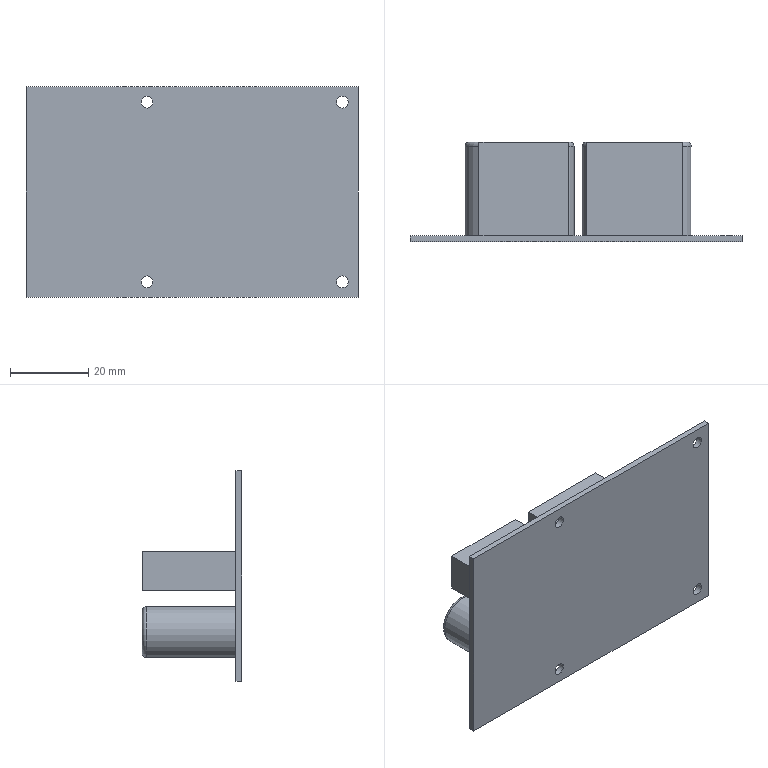Part | STEP file | 6151212W | 1 solid | 42 faces | box 85 x 25.5 x 54 mm | volume 22602 mm3 | plane 30 | cylinder 8 | torus 4 | commonest cylinder face diameters 3 x4 13 x4
STEP:
#1=CARTESIAN_POINT('',(8.051,1.5,-7.857));
#2=VERTEX_POINT('',#1);
#3=CARTESIAN_POINT('',(8.051,1.5,-14.357));
#4=DIRECTION('',(0.,1.,0.));
#5=DIRECTION('',(0.,0.,1.));
#6=AXIS2_PLACEMENT_3D('',#3,#4,#5);
#7=CIRCLE('',#6,6.5);
#8=EDGE_CURVE('',#2,#2,#7,.T.);
#9=ORIENTED_EDGE('',*,*,#8,.F.);
#10=EDGE_LOOP('',(#9));
#11=FACE_BOUND('',#10,.T.);
#12=CARTESIAN_POINT('',(-24.841,1.5,6.301));
#13=VERTEX_POINT('',#12);
#14=CARTESIAN_POINT('',(-1.911,1.5,6.301));
#15=VERTEX_POINT('',#14);
#16=CARTESIAN_POINT('',(-24.841,1.5,6.301));
#17=DIRECTION('',(1.,0.,0.));
#18=VECTOR('',#17,1000.);
#19=LINE('',#16,#18);
#20=EDGE_CURVE('',#13,#15,#19,.T.);
#21=ORIENTED_EDGE('',*,*,#20,.F.);
#22=CARTESIAN_POINT('',(-24.841,1.5,-3.718));
#23=VERTEX_POINT('',#22);
#24=CARTESIAN_POINT('',(-24.841,1.5,-3.718));
#25=DIRECTION('',(0.,0.,1.));
#26=VECTOR('',#25,1000.);
#27=LINE('',#24,#26);
#28=EDGE_CURVE('',#23,#13,#27,.T.);
#29=ORIENTED_EDGE('',*,*,#28,.F.);
#30=CARTESIAN_POINT('',(-1.911,1.5,-3.718));
#31=VERTEX_POINT('',#30);
#32=CARTESIAN_POINT('',(-24.841,1.5,-3.718));
#33=DIRECTION('',(-1.,0.,0.));
#34=VECTOR('',#33,1000.);
#35=LINE('',#32,#34);
#36=EDGE_CURVE('',#31,#23,#35,.T.);
#37=ORIENTED_EDGE('',*,*,#36,.F.);
#38=CARTESIAN_POINT('',(-1.911,1.5,-3.718));
#39=DIRECTION('',(0.,0.,-1.));
#40=VECTOR('',#39,1000.);
#41=LINE('',#38,#40);
#42=EDGE_CURVE('',#15,#31,#41,.T.);
#43=ORIENTED_EDGE('',*,*,#42,.F.);
#44=EDGE_LOOP('',(#21,#29,#37,#43));
#45=FACE_BOUND('',#44,.T.);
#46=CARTESIAN_POINT('',(-21.949,1.5,-7.857));
#47=VERTEX_POINT('',#46);
#48=CARTESIAN_POINT('',(-21.949,1.5,-14.357));
#49=DIRECTION('',(0.,1.,0.));
#50=DIRECTION('',(0.,0.,1.));
#51=AXIS2_PLACEMENT_3D('',#48,#49,#50);
#52=CIRCLE('',#51,6.5);
#53=EDGE_CURVE('',#47,#47,#52,.T.);
#54=ORIENTED_EDGE('',*,*,#53,.F.);
#55=EDGE_LOOP('',(#54));
#56=FACE_BOUND('',#55,.T.);
#57=CARTESIAN_POINT('',(38.5,1.5,21.5));
#58=VERTEX_POINT('',#57);
#59=CARTESIAN_POINT('',(38.5,1.5,23.));
#60=DIRECTION('',(0.,1.,0.));
#61=DIRECTION('',(0.,0.,-1.));
#62=AXIS2_PLACEMENT_3D('',#59,#60,#61);
#63=CIRCLE('',#62,1.5);
#64=EDGE_CURVE('',#58,#58,#63,.T.);
#65=ORIENTED_EDGE('',*,*,#64,.F.);
#66=EDGE_LOOP('',(#65));
#67=FACE_BOUND('',#66,.T.);
#68=CARTESIAN_POINT('',(-11.5,1.5,-21.5));
#69=VERTEX_POINT('',#68);
#70=CARTESIAN_POINT('',(-11.5,1.5,-23.));
#71=DIRECTION('',(0.,1.,0.));
#72=DIRECTION('',(0.,0.,1.));
#73=AXIS2_PLACEMENT_3D('',#70,#71,#72);
#74=CIRCLE('',#73,1.5);
#75=EDGE_CURVE('',#69,#69,#74,.T.);
#76=ORIENTED_EDGE('',*,*,#75,.F.);
#77=EDGE_LOOP('',(#76));
#78=FACE_BOUND('',#77,.T.);
#79=CARTESIAN_POINT('',(-42.5,1.5,-27.));
#80=VERTEX_POINT('',#79);
#81=CARTESIAN_POINT('',(-42.5,1.5,27.));
#82=VERTEX_POINT('',#81);
#83=CARTESIAN_POINT('',(-42.5,1.5,-27.));
#84=DIRECTION('',(0.,0.,1.));
#85=VECTOR('',#84,1000.);
#86=LINE('',#83,#85);
#87=EDGE_CURVE('',#80,#82,#86,.T.);
#88=ORIENTED_EDGE('',*,*,#87,.T.);
#89=CARTESIAN_POINT('',(42.5,1.5,27.));
#90=VERTEX_POINT('',#89);
#91=CARTESIAN_POINT('',(-42.5,1.5,27.));
#92=DIRECTION('',(1.,0.,0.));
#93=VECTOR('',#92,1000.);
#94=LINE('',#91,#93);
#95=EDGE_CURVE('',#82,#90,#94,.T.);
#96=ORIENTED_EDGE('',*,*,#95,.T.);
#97=CARTESIAN_POINT('',(42.5,1.5,-27.));
#98=VERTEX_POINT('',#97);
#99=CARTESIAN_POINT('',(42.5,1.5,-27.));
#100=DIRECTION('',(0.,0.,-1.));
#101=VECTOR('',#100,1000.);
#102=LINE('',#99,#101);
#103=EDGE_CURVE('',#90,#98,#102,.T.);
#104=ORIENTED_EDGE('',*,*,#103,.T.);
#105=CARTESIAN_POINT('',(-42.5,1.5,-27.));
#106=DIRECTION('',(-1.,0.,0.));
#107=VECTOR('',#106,1000.);
#108=LINE('',#105,#107);
#109=EDGE_CURVE('',#98,#80,#108,.T.);
#110=ORIENTED_EDGE('',*,*,#109,.T.);
#111=EDGE_LOOP('',(#88,#96,#104,#110));
#112=FACE_OUTER_BOUND('',#111,.T.);
#113=CARTESIAN_POINT('',(-11.5,1.5,24.5));
#114=VERTEX_POINT('',#113);
#115=CARTESIAN_POINT('',(-11.5,1.5,23.));
#116=DIRECTION('',(0.,1.,0.));
#117=DIRECTION('',(0.,0.,1.));
#118=AXIS2_PLACEMENT_3D('',#115,#116,#117);
#119=CIRCLE('',#118,1.5);
#120=EDGE_CURVE('',#114,#114,#119,.T.);
#121=ORIENTED_EDGE('',*,*,#120,.F.);
#122=EDGE_LOOP('',(#121));
#123=FACE_BOUND('',#122,.T.);
#124=CARTESIAN_POINT('',(38.5,1.5,-24.5));
#125=VERTEX_POINT('',#124);
#126=CARTESIAN_POINT('',(38.5,1.5,-23.));
#127=DIRECTION('',(0.,1.,0.));
#128=DIRECTION('',(0.,0.,-1.));
#129=AXIS2_PLACEMENT_3D('',#126,#127,#128);
#130=CIRCLE('',#129,1.5);
#131=EDGE_CURVE('',#125,#125,#130,.T.);
#132=ORIENTED_EDGE('',*,*,#131,.F.);
#133=EDGE_LOOP('',(#132));
#134=FACE_BOUND('',#133,.T.);
#135=CARTESIAN_POINT('',(-6.949,1.5,-7.857));
#136=VERTEX_POINT('',#135);
#137=CARTESIAN_POINT('',(-6.949,1.5,-14.357));
#138=DIRECTION('',(0.,1.,0.));
#139=DIRECTION('',(0.,0.,1.));
#140=AXIS2_PLACEMENT_3D('',#137,#138,#139);
#141=CIRCLE('',#140,6.5);
#142=EDGE_CURVE('',#136,#136,#141,.T.);
#143=ORIENTED_EDGE('',*,*,#142,.F.);
#144=EDGE_LOOP('',(#143));
#145=FACE_BOUND('',#144,.T.);
#146=CARTESIAN_POINT('',(23.051,1.5,-7.857));
#147=VERTEX_POINT('',#146);
#148=CARTESIAN_POINT('',(23.051,1.5,-14.357));
#149=DIRECTION('',(0.,1.,0.));
#150=DIRECTION('',(0.,0.,1.));
#151=AXIS2_PLACEMENT_3D('',#148,#149,#150);
#152=CIRCLE('',#151,6.5);
#153=EDGE_CURVE('',#147,#147,#152,.T.);
#154=ORIENTED_EDGE('',*,*,#153,.F.);
#155=EDGE_LOOP('',(#154));
#156=FACE_BOUND('',#155,.T.);
#157=CARTESIAN_POINT('',(2.737,1.5,6.301));
#158=VERTEX_POINT('',#157);
#159=CARTESIAN_POINT('',(27.32,1.5,6.301));
#160=VERTEX_POINT('',#159);
#161=CARTESIAN_POINT('',(2.737,1.5,6.301));
#162=DIRECTION('',(1.,0.,0.));
#163=VECTOR('',#162,1000.);
#164=LINE('',#161,#163);
#165=EDGE_CURVE('',#158,#160,#164,.T.);
#166=ORIENTED_EDGE('',*,*,#165,.F.);
#167=CARTESIAN_POINT('',(2.737,1.5,-3.718));
#168=VERTEX_POINT('',#167);
#169=CARTESIAN_POINT('',(2.737,1.5,-3.718));
#170=DIRECTION('',(0.,0.,1.));
#171=VECTOR('',#170,1000.);
#172=LINE('',#169,#171);
#173=EDGE_CURVE('',#168,#158,#172,.T.);
#174=ORIENTED_EDGE('',*,*,#173,.F.);
#175=CARTESIAN_POINT('',(27.32,1.5,-3.718));
#176=VERTEX_POINT('',#175);
#177=CARTESIAN_POINT('',(2.737,1.5,-3.718));
#178=DIRECTION('',(-1.,0.,0.));
#179=VECTOR('',#178,1000.);
#180=LINE('',#177,#179);
#181=EDGE_CURVE('',#176,#168,#180,.T.);
#182=ORIENTED_EDGE('',*,*,#181,.F.);
#183=CARTESIAN_POINT('',(27.32,1.5,-3.718));
#184=DIRECTION('',(0.,0.,-1.));
#185=VECTOR('',#184,1000.);
#186=LINE('',#183,#185);
#187=EDGE_CURVE('',#160,#176,#186,.T.);
#188=ORIENTED_EDGE('',*,*,#187,.F.);
#189=EDGE_LOOP('',(#166,#174,#182,#188));
#190=FACE_BOUND('',#189,.T.);
#191=CARTESIAN_POINT('',(-42.5,1.5,-27.));
#192=DIRECTION('',(0.,1.,0.));
#193=DIRECTION('',(0.,0.,1.));
#194=AXIS2_PLACEMENT_3D('',#191,#192,#193);
#195=PLANE('',#194);
#196=ADVANCED_FACE('',(#11,#45,#56,#67,#78,#112,#123,#134,#145,#156,#190),#195,.T.);
#197=CARTESIAN_POINT('',(38.5,0.,21.5));
#198=VERTEX_POINT('',#197);
#199=CARTESIAN_POINT('',(38.5,0.,23.));
#200=DIRECTION('',(0.,1.,0.));
#201=DIRECTION('',(0.,0.,-1.));
#202=AXIS2_PLACEMENT_3D('',#199,#200,#201);
#203=CIRCLE('',#202,1.5);
#204=EDGE_CURVE('',#198,#198,#203,.T.);
#205=ORIENTED_EDGE('',*,*,#204,.T.);
#206=EDGE_LOOP('',(#205));
#207=FACE_BOUND('',#206,.T.);
#208=CARTESIAN_POINT('',(-11.5,0.,-21.5));
#209=VERTEX_POINT('',#208);
#210=CARTESIAN_POINT('',(-11.5,0.,-23.));
#211=DIRECTION('',(0.,1.,0.));
#212=DIRECTION('',(0.,0.,1.));
#213=AXIS2_PLACEMENT_3D('',#210,#211,#212);
#214=CIRCLE('',#213,1.5);
#215=EDGE_CURVE('',#209,#209,#214,.T.);
#216=ORIENTED_EDGE('',*,*,#215,.T.);
#217=EDGE_LOOP('',(#216));
#218=FACE_BOUND('',#217,.T.);
#219=CARTESIAN_POINT('',(-42.5,0.,-27.));
#220=VERTEX_POINT('',#219);
#221=CARTESIAN_POINT('',(-42.5,0.,27.));
#222=VERTEX_POINT('',#221);
#223=CARTESIAN_POINT('',(-42.5,0.,-27.));
#224=DIRECTION('',(0.,0.,1.));
#225=VECTOR('',#224,1000.);
#226=LINE('',#223,#225);
#227=EDGE_CURVE('',#220,#222,#226,.T.);
#228=ORIENTED_EDGE('',*,*,#227,.F.);
#229=CARTESIAN_POINT('',(42.5,0.,-27.));
#230=VERTEX_POINT('',#229);
#231=CARTESIAN_POINT('',(-42.5,0.,-27.));
#232=DIRECTION('',(-1.,0.,0.));
#233=VECTOR('',#232,1000.);
#234=LINE('',#231,#233);
#235=EDGE_CURVE('',#230,#220,#234,.T.);
#236=ORIENTED_EDGE('',*,*,#235,.F.);
#237=CARTESIAN_POINT('',(42.5,0.,27.));
#238=VERTEX_POINT('',#237);
#239=CARTESIAN_POINT('',(42.5,0.,-27.));
#240=DIRECTION('',(0.,0.,-1.));
#241=VECTOR('',#240,1000.);
#242=LINE('',#239,#241);
#243=EDGE_CURVE('',#238,#230,#242,.T.);
#244=ORIENTED_EDGE('',*,*,#243,.F.);
#245=CARTESIAN_POINT('',(-42.5,0.,27.));
#246=DIRECTION('',(1.,0.,0.));
#247=VECTOR('',#246,1000.);
#248=LINE('',#245,#247);
#249=EDGE_CURVE('',#222,#238,#248,.T.);
#250=ORIENTED_EDGE('',*,*,#249,.F.);
#251=EDGE_LOOP('',(#228,#236,#244,#250));
#252=FACE_OUTER_BOUND('',#251,.T.);
#253=CARTESIAN_POINT('',(-11.5,0.,24.5));
#254=VERTEX_POINT('',#253);
#255=CARTESIAN_POINT('',(-11.5,0.,23.));
#256=DIRECTION('',(0.,1.,0.));
#257=DIRECTION('',(0.,0.,1.));
#258=AXIS2_PLACEMENT_3D('',#255,#256,#257);
#259=CIRCLE('',#258,1.5);
#260=EDGE_CURVE('',#254,#254,#259,.T.);
#261=ORIENTED_EDGE('',*,*,#260,.T.);
#262=EDGE_LOOP('',(#261));
#263=FACE_BOUND('',#262,.T.);
#264=CARTESIAN_POINT('',(38.5,0.,-24.5));
#265=VERTEX_POINT('',#264);
#266=CARTESIAN_POINT('',(38.5,0.,-23.));
#267=DIRECTION('',(0.,1.,0.));
#268=DIRECTION('',(0.,0.,-1.));
#269=AXIS2_PLACEMENT_3D('',#266,#267,#268);
#270=CIRCLE('',#269,1.5);
#271=EDGE_CURVE('',#265,#265,#270,.T.);
#272=ORIENTED_EDGE('',*,*,#271,.T.);
#273=EDGE_LOOP('',(#272));
#274=FACE_BOUND('',#273,.T.);
#275=CARTESIAN_POINT('',(-42.5,0.,-27.));
#276=DIRECTION('',(0.,1.,0.));
#277=DIRECTION('',(0.,0.,1.));
#278=AXIS2_PLACEMENT_3D('',#275,#276,#277);
#279=PLANE('',#278);
#280=ADVANCED_FACE('',(#207,#218,#252,#263,#274),#279,.F.);
#281=ORIENTED_EDGE('',*,*,#227,.T.);
#282=CARTESIAN_POINT('',(-42.5,1.5,27.));
#283=DIRECTION('',(0.,-1.,0.));
#284=VECTOR('',#283,1000.);
#285=LINE('',#282,#284);
#286=EDGE_CURVE('',#82,#222,#285,.T.);
#287=ORIENTED_EDGE('',*,*,#286,.F.);
#288=ORIENTED_EDGE('',*,*,#87,.F.);
#289=CARTESIAN_POINT('',(-42.5,1.5,-27.));
#290=DIRECTION('',(0.,-1.,0.));
#291=VECTOR('',#290,1000.);
#292=LINE('',#289,#291);
#293=EDGE_CURVE('',#80,#220,#292,.T.);
#294=ORIENTED_EDGE('',*,*,#293,.T.);
#295=EDGE_LOOP('',(#281,#287,#288,#294));
#296=FACE_OUTER_BOUND('',#295,.T.);
#297=CARTESIAN_POINT('',(-42.5,1.5,-27.));
#298=DIRECTION('',(1.,0.,0.));
#299=DIRECTION('',(0.,0.,-1.));
#300=AXIS2_PLACEMENT_3D('',#297,#298,#299);
#301=PLANE('',#300);
#302=ADVANCED_FACE('',(#296),#301,.F.);
#303=ORIENTED_EDGE('',*,*,#249,.T.);
#304=CARTESIAN_POINT('',(42.5,1.5,27.));
#305=DIRECTION('',(0.,-1.,0.));
#306=VECTOR('',#305,1000.);
#307=LINE('',#304,#306);
#308=EDGE_CURVE('',#90,#238,#307,.T.);
#309=ORIENTED_EDGE('',*,*,#308,.F.);
#310=ORIENTED_EDGE('',*,*,#95,.F.);
#311=ORIENTED_EDGE('',*,*,#286,.T.);
#312=EDGE_LOOP('',(#303,#309,#310,#311));
#313=FACE_OUTER_BOUND('',#312,.T.);
#314=CARTESIAN_POINT('',(-42.5,1.5,27.));
#315=DIRECTION('',(0.,0.,-1.));
#316=DIRECTION('',(-1.,0.,0.));
#317=AXIS2_PLACEMENT_3D('',#314,#315,#316);
#318=PLANE('',#317);
#319=ADVANCED_FACE('',(#313),#318,.F.);
#320=ORIENTED_EDGE('',*,*,#243,.T.);
#321=CARTESIAN_POINT('',(42.5,1.5,-27.));
#322=DIRECTION('',(0.,-1.,0.));
#323=VECTOR('',#322,1000.);
#324=LINE('',#321,#323);
#325=EDGE_CURVE('',#98,#230,#324,.T.);
#326=ORIENTED_EDGE('',*,*,#325,.F.);
#327=ORIENTED_EDGE('',*,*,#103,.F.);
#328=ORIENTED_EDGE('',*,*,#308,.T.);
#329=EDGE_LOOP('',(#320,#326,#327,#328));
#330=FACE_OUTER_BOUND('',#329,.T.);
#331=CARTESIAN_POINT('',(42.5,1.5,-27.));
#332=DIRECTION('',(-1.,0.,0.));
#333=DIRECTION('',(0.,0.,1.));
#334=AXIS2_PLACEMENT_3D('',#331,#332,#333);
#335=PLANE('',#334);
#336=ADVANCED_FACE('',(#330),#335,.F.);
#337=ORIENTED_EDGE('',*,*,#235,.T.);
#338=ORIENTED_EDGE('',*,*,#293,.F.);
#339=ORIENTED_EDGE('',*,*,#109,.F.);
#340=ORIENTED_EDGE('',*,*,#325,.T.);
#341=EDGE_LOOP('',(#337,#338,#339,#340));
#342=FACE_OUTER_BOUND('',#341,.T.);
#343=CARTESIAN_POINT('',(-42.5,1.5,-27.));
#344=DIRECTION('',(0.,0.,1.));
#345=DIRECTION('',(1.,0.,0.));
#346=AXIS2_PLACEMENT_3D('',#343,#344,#345);
#347=PLANE('',#346);
#348=ADVANCED_FACE('',(#342),#347,.F.);
#349=ORIENTED_EDGE('',*,*,#75,.T.);
#350=EDGE_LOOP('',(#349));
#351=FACE_OUTER_BOUND('',#350,.T.);
#352=ORIENTED_EDGE('',*,*,#215,.F.);
#353=EDGE_LOOP('',(#352));
#354=FACE_OUTER_BOUND('',#353,.T.);
#355=CARTESIAN_POINT('',(-11.5,1.5,-23.));
#356=DIRECTION('',(0.,-1.,0.));
#357=DIRECTION('',(0.,0.,-1.));
#358=AXIS2_PLACEMENT_3D('',#355,#356,#357);
#359=CYLINDRICAL_SURFACE('',#358,1.5);
#360=ADVANCED_FACE('',(#351,#354),#359,.F.);
#361=ORIENTED_EDGE('',*,*,#120,.T.);
#362=EDGE_LOOP('',(#361));
#363=FACE_OUTER_BOUND('',#362,.T.);
#364=ORIENTED_EDGE('',*,*,#260,.F.);
#365=EDGE_LOOP('',(#364));
#366=FACE_OUTER_BOUND('',#365,.T.);
#367=CARTESIAN_POINT('',(-11.5,1.5,23.));
#368=DIRECTION('',(0.,-1.,0.));
#369=DIRECTION('',(0.,0.,-1.));
#370=AXIS2_PLACEMENT_3D('',#367,#368,#369);
#371=CYLINDRICAL_SURFACE('',#370,1.5);
#372=ADVANCED_FACE('',(#363,#366),#371,.F.);
#373=ORIENTED_EDGE('',*,*,#64,.T.);
#374=EDGE_LOOP('',(#373));
#375=FACE_OUTER_BOUND('',#374,.T.);
#376=ORIENTED_EDGE('',*,*,#204,.F.);
#377=EDGE_LOOP('',(#376));
#378=FACE_OUTER_BOUND('',#377,.T.);
#379=CARTESIAN_POINT('',(38.5,1.5,23.));
#380=DIRECTION('',(0.,-1.,0.));
#381=DIRECTION('',(0.,0.,-1.));
#382=AXIS2_PLACEMENT_3D('',#379,#380,#381);
#383=CYLINDRICAL_SURFACE('',#382,1.5);
#384=ADVANCED_FACE('',(#375,#378),#383,.F.);
#385=ORIENTED_EDGE('',*,*,#131,.T.);
#386=EDGE_LOOP('',(#385));
#387=FACE_OUTER_BOUND('',#386,.T.);
#388=ORIENTED_EDGE('',*,*,#271,.F.);
#389=EDGE_LOOP('',(#388));
#390=FACE_OUTER_BOUND('',#389,.T.);
#391=CARTESIAN_POINT('',(38.5,1.5,-23.));
#392=DIRECTION('',(0.,-1.,0.));
#393=DIRECTION('',(0.,0.,-1.));
#394=AXIS2_PLACEMENT_3D('',#391,#392,#393);
#395=CYLINDRICAL_SURFACE('',#394,1.5);
#396=ADVANCED_FACE('',(#387,#390),#395,.F.);
#397=CARTESIAN_POINT('',(-21.949,24.5,-7.857));
#398=VERTEX_POINT('',#397);
#399=CARTESIAN_POINT('',(-21.949,24.5,-14.357));
#400=DIRECTION('',(0.,-1.,0.));
#401=DIRECTION('',(0.,0.,1.));
#402=AXIS2_PLACEMENT_3D('',#399,#400,#401);
#403=CIRCLE('',#402,6.5);
#404=EDGE_CURVE('',#398,#398,#403,.T.);
#405=ORIENTED_EDGE('',*,*,#404,.T.);
#406=EDGE_LOOP('',(#405));
#407=FACE_OUTER_BOUND('',#406,.T.);
#408=ORIENTED_EDGE('',*,*,#53,.T.);
#409=EDGE_LOOP('',(#408));
#410=FACE_OUTER_BOUND('',#409,.T.);
#411=CARTESIAN_POINT('',(-21.949,25.5,-14.357));
#412=DIRECTION('',(0.,-1.,0.));
#413=DIRECTION('',(0.,0.,-1.));
#414=AXIS2_PLACEMENT_3D('',#411,#412,#413);
#415=CYLINDRICAL_SURFACE('',#414,6.5);
#416=ADVANCED_FACE('',(#407,#410),#415,.T.);
#417=CARTESIAN_POINT('',(-21.949,25.5,-8.857));
#418=VERTEX_POINT('',#417);
#419=CARTESIAN_POINT('',(-21.949,25.5,-14.357));
#420=DIRECTION('',(0.,1.,0.));
#421=DIRECTION('',(0.,0.,1.));
#422=AXIS2_PLACEMENT_3D('',#419,#420,#421);
#423=CIRCLE('',#422,5.5);
#424=EDGE_CURVE('',#418,#418,#423,.T.);
#425=ORIENTED_EDGE('',*,*,#424,.T.);
#426=EDGE_LOOP('',(#425));
#427=FACE_OUTER_BOUND('',#426,.T.);
#428=CARTESIAN_POINT('',(-21.949,25.5,-14.357));
#429=DIRECTION('',(0.,1.,0.));
#430=DIRECTION('',(0.,0.,1.));
#431=AXIS2_PLACEMENT_3D('',#428,#429,#430);
#432=PLANE('',#431);
#433=ADVANCED_FACE('',(#427),#432,.T.);
#434=CARTESIAN_POINT('',(-24.841,25.5,-3.718));
#435=VERTEX_POINT('',#434);
#436=CARTESIAN_POINT('',(-24.841,25.5,6.301));
#437=VERTEX_POINT('',#436);
#438=CARTESIAN_POINT('',(-24.841,25.5,-3.718));
#439=DIRECTION('',(0.,0.,1.));
#440=VECTOR('',#439,1000.);
#441=LINE('',#438,#440);
#442=EDGE_CURVE('',#435,#437,#441,.T.);
#443=ORIENTED_EDGE('',*,*,#442,.T.);
#444=CARTESIAN_POINT('',(-1.911,25.5,6.301));
#445=VERTEX_POINT('',#444);
#446=CARTESIAN_POINT('',(-24.841,25.5,6.301));
#447=DIRECTION('',(1.,0.,0.));
#448=VECTOR('',#447,1000.);
#449=LINE('',#446,#448);
#450=EDGE_CURVE('',#437,#445,#449,.T.);
#451=ORIENTED_EDGE('',*,*,#450,.T.);
#452=CARTESIAN_POINT('',(-1.911,25.5,-3.718));
#453=VERTEX_POINT('',#452);
#454=CARTESIAN_POINT('',(-1.911,25.5,-3.718));
#455=DIRECTION('',(0.,0.,-1.));
#456=VECTOR('',#455,1000.);
#457=LINE('',#454,#456);
#458=EDGE_CURVE('',#445,#453,#457,.T.);
#459=ORIENTED_EDGE('',*,*,#458,.T.);
#460=CARTESIAN_POINT('',(-24.841,25.5,-3.718));
#461=DIRECTION('',(-1.,0.,0.));
#462=VECTOR('',#461,1000.);
#463=LINE('',#460,#462);
#464=EDGE_CURVE('',#453,#435,#463,.T.);
#465=ORIENTED_EDGE('',*,*,#464,.T.);
#466=EDGE_LOOP('',(#443,#451,#459,#465));
#467=FACE_OUTER_BOUND('',#466,.T.);
#468=CARTESIAN_POINT('',(-23.841,25.5,5.301));
#469=VERTEX_POINT('',#468);
#470=CARTESIAN_POINT('',(-2.911,25.5,5.301));
#471=VERTEX_POINT('',#470);
#472=CARTESIAN_POINT('',(-23.841,25.5,5.301));
#473=DIRECTION('',(1.,0.,0.));
#474=VECTOR('',#473,1000.);
#475=LINE('',#472,#474);
#476=EDGE_CURVE('',#469,#471,#475,.T.);
#477=ORIENTED_EDGE('',*,*,#476,.F.);
#478=CARTESIAN_POINT('',(-23.841,25.5,-2.718));
#479=VERTEX_POINT('',#478);
#480=CARTESIAN_POINT('',(-23.841,25.5,-2.718));
#481=DIRECTION('',(0.,0.,1.));
#482=VECTOR('',#481,1000.);
#483=LINE('',#480,#482);
#484=EDGE_CURVE('',#479,#469,#483,.T.);
#485=ORIENTED_EDGE('',*,*,#484,.F.);
#486=CARTESIAN_POINT('',(-2.911,25.5,-2.718));
#487=VERTEX_POINT('',#486);
#488=CARTESIAN_POINT('',(-23.841,25.5,-2.718));
#489=DIRECTION('',(-1.,0.,0.));
#490=VECTOR('',#489,1000.);
#491=LINE('',#488,#490);
#492=EDGE_CURVE('',#487,#479,#491,.T.);
#493=ORIENTED_EDGE('',*,*,#492,.F.);
#494=CARTESIAN_POINT('',(-2.911,25.5,-2.718));
#495=DIRECTION('',(0.,0.,-1.));
#496=VECTOR('',#495,1000.);
#497=LINE('',#494,#496);
#498=EDGE_CURVE('',#471,#487,#497,.T.);
#499=ORIENTED_EDGE('',*,*,#498,.F.);
#500=EDGE_LOOP('',(#477,#485,#493,#499));
#501=FACE_BOUND('',#500,.T.);
#502=CARTESIAN_POINT('',(-24.841,25.5,6.301));
#503=DIRECTION('',(0.,1.,0.));
#504=DIRECTION('',(0.,0.,1.));
#505=AXIS2_PLACEMENT_3D('',#502,#503,#504);
#506=PLANE('',#505);
#507=ADVANCED_FACE('',(#467,#501),#506,.T.);
#508=ORIENTED_EDGE('',*,*,#28,.T.);
#509=CARTESIAN_POINT('',(-24.841,25.5,6.301));
#510=DIRECTION('',(0.,-1.,0.));
#511=VECTOR('',#510,1000.);
#512=LINE('',#509,#511);
#513=EDGE_CURVE('',#437,#13,#512,.T.);
#514=ORIENTED_EDGE('',*,*,#513,.F.);
#515=ORIENTED_EDGE('',*,*,#442,.F.);
#516=CARTESIAN_POINT('',(-24.841,25.5,-3.718));
#517=DIRECTION('',(0.,-1.,0.));
#518=VECTOR('',#517,1000.);
#519=LINE('',#516,#518);
#520=EDGE_CURVE('',#435,#23,#519,.T.);
#521=ORIENTED_EDGE('',*,*,#520,.T.);
#522=EDGE_LOOP('',(#508,#514,#515,#521));
#523=FACE_OUTER_BOUND('',#522,.T.);
#524=CARTESIAN_POINT('',(-24.841,25.5,-3.718));
#525=DIRECTION('',(1.,0.,0.));
#526=DIRECTION('',(0.,0.,-1.));
#527=AXIS2_PLACEMENT_3D('',#524,#525,#526);
#528=PLANE('',#527);
#529=ADVANCED_FACE('',(#523),#528,.F.);
#530=ORIENTED_EDGE('',*,*,#20,.T.);
#531=CARTESIAN_POINT('',(-1.911,25.5,6.301));
#532=DIRECTION('',(0.,-1.,0.));
#533=VECTOR('',#532,1000.);
#534=LINE('',#531,#533);
#535=EDGE_CURVE('',#445,#15,#534,.T.);
#536=ORIENTED_EDGE('',*,*,#535,.F.);
#537=ORIENTED_EDGE('',*,*,#450,.F.);
#538=ORIENTED_EDGE('',*,*,#513,.T.);
#539=EDGE_LOOP('',(#530,#536,#537,#538));
#540=FACE_OUTER_BOUND('',#539,.T.);
#541=CARTESIAN_POINT('',(-24.841,25.5,6.301));
#542=DIRECTION('',(0.,0.,-1.));
#543=DIRECTION('',(-1.,0.,0.));
#544=AXIS2_PLACEMENT_3D('',#541,#542,#543);
#545=PLANE('',#544);
#546=ADVANCED_FACE('',(#540),#545,.F.);
#547=ORIENTED_EDGE('',*,*,#42,.T.);
#548=CARTESIAN_POINT('',(-1.911,25.5,-3.718));
#549=DIRECTION('',(0.,-1.,0.));
#550=VECTOR('',#549,1000.);
#551=LINE('',#548,#550);
#552=EDGE_CURVE('',#453,#31,#551,.T.);
#553=ORIENTED_EDGE('',*,*,#552,.F.);
#554=ORIENTED_EDGE('',*,*,#458,.F.);
#555=ORIENTED_EDGE('',*,*,#535,.T.);
#556=EDGE_LOOP('',(#547,#553,#554,#555));
#557=FACE_OUTER_BOUND('',#556,.T.);
#558=CARTESIAN_POINT('',(-1.911,25.5,-3.718));
#559=DIRECTION('',(-1.,0.,0.));
#560=DIRECTION('',(0.,0.,1.));
#561=AXIS2_PLACEMENT_3D('',#558,#559,#560);
#562=PLANE('',#561);
#563=ADVANCED_FACE('',(#557),#562,.F.);
#564=ORIENTED_EDGE('',*,*,#36,.T.);
#565=ORIENTED_EDGE('',*,*,#520,.F.);
#566=ORIENTED_EDGE('',*,*,#464,.F.);
#567=ORIENTED_EDGE('',*,*,#552,.T.);
#568=EDGE_LOOP('',(#564,#565,#566,#567));
#569=FACE_OUTER_BOUND('',#568,.T.);
#570=CARTESIAN_POINT('',(-24.841,25.5,-3.718));
#571=DIRECTION('',(0.,0.,1.));
#572=DIRECTION('',(1.,0.,0.));
#573=AXIS2_PLACEMENT_3D('',#570,#571,#572);
#574=PLANE('',#573);
#575=ADVANCED_FACE('',(#569),#574,.F.);
#576=CARTESIAN_POINT('',(-23.841,1.5,-2.718));
#577=VERTEX_POINT('',#576);
#578=CARTESIAN_POINT('',(-23.841,1.5,5.301));
#579=VERTEX_POINT('',#578);
#580=CARTESIAN_POINT('',(-23.841,1.5,-2.718));
#581=DIRECTION('',(0.,0.,1.));
#582=VECTOR('',#581,1000.);
#583=LINE('',#580,#582);
#584=EDGE_CURVE('',#577,#579,#583,.T.);
#585=ORIENTED_EDGE('',*,*,#584,.F.);
#586=CARTESIAN_POINT('',(-23.841,25.5,-2.718));
#587=DIRECTION('',(0.,-1.,0.));
#588=VECTOR('',#587,1000.);
#589=LINE('',#586,#588);
#590=EDGE_CURVE('',#479,#577,#589,.T.);
#591=ORIENTED_EDGE('',*,*,#590,.F.);
#592=ORIENTED_EDGE('',*,*,#484,.T.);
#593=CARTESIAN_POINT('',(-23.841,25.5,5.301));
#594=DIRECTION('',(0.,-1.,0.));
#595=VECTOR('',#594,1000.);
#596=LINE('',#593,#595);
#597=EDGE_CURVE('',#469,#579,#596,.T.);
#598=ORIENTED_EDGE('',*,*,#597,.T.);
#599=EDGE_LOOP('',(#585,#591,#592,#598));
#600=FACE_OUTER_BOUND('',#599,.T.);
#601=CARTESIAN_POINT('',(-23.841,25.5,-2.718));
#602=DIRECTION('',(1.,0.,0.));
#603=DIRECTION('',(0.,0.,-1.));
#604=AXIS2_PLACEMENT_3D('',#601,#602,#603);
#605=PLANE('',#604);
#606=ADVANCED_FACE('',(#600),#605,.T.);
#607=CARTESIAN_POINT('',(-2.911,1.5,5.301));
#608=VERTEX_POINT('',#607);
#609=CARTESIAN_POINT('',(-23.841,1.5,5.301));
#610=DIRECTION('',(1.,0.,0.));
#611=VECTOR('',#610,1000.);
#612=LINE('',#609,#611);
#613=EDGE_CURVE('',#579,#608,#612,.T.);
#614=ORIENTED_EDGE('',*,*,#613,.F.);
#615=ORIENTED_EDGE('',*,*,#597,.F.);
#616=ORIENTED_EDGE('',*,*,#476,.T.);
#617=CARTESIAN_POINT('',(-2.911,25.5,5.301));
#618=DIRECTION('',(0.,-1.,0.));
#619=VECTOR('',#618,1000.);
#620=LINE('',#617,#619);
#621=EDGE_CURVE('',#471,#608,#620,.T.);
#622=ORIENTED_EDGE('',*,*,#621,.T.);
#623=EDGE_LOOP('',(#614,#615,#616,#622));
#624=FACE_OUTER_BOUND('',#623,.T.);
#625=CARTESIAN_POINT('',(-23.841,25.5,5.301));
#626=DIRECTION('',(0.,0.,-1.));
#627=DIRECTION('',(-1.,0.,0.));
#628=AXIS2_PLACEMENT_3D('',#625,#626,#627);
#629=PLANE('',#628);
#630=ADVANCED_FACE('',(#624),#629,.T.);
#631=CARTESIAN_POINT('',(-2.911,1.5,-2.718));
#632=VERTEX_POINT('',#631);
#633=CARTESIAN_POINT('',(-2.911,1.5,-2.718));
#634=DIRECTION('',(0.,0.,-1.));
#635=VECTOR('',#634,1000.);
#636=LINE('',#633,#635);
#637=EDGE_CURVE('',#608,#632,#636,.T.);
#638=ORIENTED_EDGE('',*,*,#637,.F.);
#639=ORIENTED_EDGE('',*,*,#621,.F.);
#640=ORIENTED_EDGE('',*,*,#498,.T.);
#641=CARTESIAN_POINT('',(-2.911,25.5,-2.718));
#642=DIRECTION('',(0.,-1.,0.));
#643=VECTOR('',#642,1000.);
#644=LINE('',#641,#643);
#645=EDGE_CURVE('',#487,#632,#644,.T.);
#646=ORIENTED_EDGE('',*,*,#645,.T.);
#647=EDGE_LOOP('',(#638,#639,#640,#646));
#648=FACE_OUTER_BOUND('',#647,.T.);
#649=CARTESIAN_POINT('',(-2.911,25.5,-2.718));
#650=DIRECTION('',(-1.,0.,0.));
#651=DIRECTION('',(0.,0.,1.));
#652=AXIS2_PLACEMENT_3D('',#649,#650,#651);
#653=PLANE('',#652);
#654=ADVANCED_FACE('',(#648),#653,.T.);
#655=CARTESIAN_POINT('',(-23.841,1.5,-2.718));
#656=DIRECTION('',(-1.,0.,0.));
#657=VECTOR('',#656,1000.);
#658=LINE('',#655,#657);
#659=EDGE_CURVE('',#632,#577,#658,.T.);
#660=ORIENTED_EDGE('',*,*,#659,.F.);
#661=ORIENTED_EDGE('',*,*,#645,.F.);
#662=ORIENTED_EDGE('',*,*,#492,.T.);
#663=ORIENTED_EDGE('',*,*,#590,.T.);
#664=EDGE_LOOP('',(#660,#661,#662,#663));
#665=FACE_OUTER_BOUND('',#664,.T.);
#666=CARTESIAN_POINT('',(-23.841,25.5,-2.718));
#667=DIRECTION('',(0.,0.,1.));
#668=DIRECTION('',(1.,0.,0.));
#669=AXIS2_PLACEMENT_3D('',#666,#667,#668);
#670=PLANE('',#669);
#671=ADVANCED_FACE('',(#665),#670,.T.);
#672=ORIENTED_EDGE('',*,*,#584,.T.);
#673=ORIENTED_EDGE('',*,*,#613,.T.);
#674=ORIENTED_EDGE('',*,*,#637,.T.);
#675=ORIENTED_EDGE('',*,*,#659,.T.);
#676=EDGE_LOOP('',(#672,#673,#674,#675));
#677=FACE_OUTER_BOUND('',#676,.T.);
#678=CARTESIAN_POINT('',(-42.5,1.5,-27.));
#679=DIRECTION('',(0.,1.,0.));
#680=DIRECTION('',(0.,0.,1.));
#681=AXIS2_PLACEMENT_3D('',#678,#679,#680);
#682=PLANE('',#681);
#683=ADVANCED_FACE('',(#677),#682,.T.);
#684=CARTESIAN_POINT('',(-6.949,24.5,-7.857));
#685=VERTEX_POINT('',#684);
#686=CARTESIAN_POINT('',(-6.949,24.5,-14.357));
#687=DIRECTION('',(0.,-1.,0.));
#688=DIRECTION('',(0.,0.,1.));
#689=AXIS2_PLACEMENT_3D('',#686,#687,#688);
#690=CIRCLE('',#689,6.5);
#691=EDGE_CURVE('',#685,#685,#690,.T.);
#692=ORIENTED_EDGE('',*,*,#691,.T.);
#693=EDGE_LOOP('',(#692));
#694=FACE_OUTER_BOUND('',#693,.T.);
#695=ORIENTED_EDGE('',*,*,#142,.T.);
#696=EDGE_LOOP('',(#695));
#697=FACE_OUTER_BOUND('',#696,.T.);
#698=CARTESIAN_POINT('',(-6.949,25.5,-14.357));
#699=DIRECTION('',(0.,-1.,0.));
#700=DIRECTION('',(0.,0.,-1.));
#701=AXIS2_PLACEMENT_3D('',#698,#699,#700);
#702=CYLINDRICAL_SURFACE('',#701,6.5);
#703=ADVANCED_FACE('',(#694,#697),#702,.T.);
#704=CARTESIAN_POINT('',(-6.949,25.5,-8.857));
#705=VERTEX_POINT('',#704);
#706=CARTESIAN_POINT('',(-6.949,25.5,-14.357));
#707=DIRECTION('',(0.,1.,0.));
#708=DIRECTION('',(0.,0.,1.));
#709=AXIS2_PLACEMENT_3D('',#706,#707,#708);
#710=CIRCLE('',#709,5.5);
#711=EDGE_CURVE('',#705,#705,#710,.T.);
#712=ORIENTED_EDGE('',*,*,#711,.T.);
#713=EDGE_LOOP('',(#712));
#714=FACE_OUTER_BOUND('',#713,.T.);
#715=CARTESIAN_POINT('',(-6.949,25.5,-14.357));
#716=DIRECTION('',(0.,1.,0.));
#717=DIRECTION('',(0.,0.,1.));
#718=AXIS2_PLACEMENT_3D('',#715,#716,#717);
#719=PLANE('',#718);
#720=ADVANCED_FACE('',(#714),#719,.T.);
#721=CARTESIAN_POINT('',(8.051,24.5,-7.857));
#722=VERTEX_POINT('',#721);
#723=CARTESIAN_POINT('',(8.051,24.5,-14.357));
#724=DIRECTION('',(0.,-1.,0.));
#725=DIRECTION('',(0.,0.,1.));
#726=AXIS2_PLACEMENT_3D('',#723,#724,#725);
#727=CIRCLE('',#726,6.5);
#728=EDGE_CURVE('',#722,#722,#727,.T.);
#729=ORIENTED_EDGE('',*,*,#728,.T.);
#730=EDGE_LOOP('',(#729));
#731=FACE_OUTER_BOUND('',#730,.T.);
#732=ORIENTED_EDGE('',*,*,#8,.T.);
#733=EDGE_LOOP('',(#732));
#734=FACE_OUTER_BOUND('',#733,.T.);
#735=CARTESIAN_POINT('',(8.051,25.5,-14.357));
#736=DIRECTION('',(0.,-1.,0.));
#737=DIRECTION('',(0.,0.,-1.));
#738=AXIS2_PLACEMENT_3D('',#735,#736,#737);
#739=CYLINDRICAL_SURFACE('',#738,6.5);
#740=ADVANCED_FACE('',(#731,#734),#739,.T.);
#741=CARTESIAN_POINT('',(8.051,25.5,-8.857));
#742=VERTEX_POINT('',#741);
#743=CARTESIAN_POINT('',(8.051,25.5,-14.357));
#744=DIRECTION('',(0.,1.,0.));
#745=DIRECTION('',(0.,0.,1.));
#746=AXIS2_PLACEMENT_3D('',#743,#744,#745);
#747=CIRCLE('',#746,5.5);
#748=EDGE_CURVE('',#742,#742,#747,.T.);
#749=ORIENTED_EDGE('',*,*,#748,.T.);
#750=EDGE_LOOP('',(#749));
#751=FACE_OUTER_BOUND('',#750,.T.);
#752=CARTESIAN_POINT('',(8.051,25.5,-14.357));
#753=DIRECTION('',(0.,1.,0.));
#754=DIRECTION('',(0.,0.,1.));
#755=AXIS2_PLACEMENT_3D('',#752,#753,#754);
#756=PLANE('',#755);
#757=ADVANCED_FACE('',(#751),#756,.T.);
#758=CARTESIAN_POINT('',(23.051,24.5,-7.857));
#759=VERTEX_POINT('',#758);
#760=CARTESIAN_POINT('',(23.051,24.5,-14.357));
#761=DIRECTION('',(0.,-1.,0.));
#762=DIRECTION('',(0.,0.,1.));
#763=AXIS2_PLACEMENT_3D('',#760,#761,#762);
#764=CIRCLE('',#763,6.5);
#765=EDGE_CURVE('',#759,#759,#764,.T.);
#766=ORIENTED_EDGE('',*,*,#765,.T.);
#767=EDGE_LOOP('',(#766));
#768=FACE_OUTER_BOUND('',#767,.T.);
#769=ORIENTED_EDGE('',*,*,#153,.T.);
#770=EDGE_LOOP('',(#769));
#771=FACE_OUTER_BOUND('',#770,.T.);
#772=CARTESIAN_POINT('',(23.051,25.5,-14.357));
#773=DIRECTION('',(0.,-1.,0.));
#774=DIRECTION('',(0.,0.,-1.));
#775=AXIS2_PLACEMENT_3D('',#772,#773,#774);
#776=CYLINDRICAL_SURFACE('',#775,6.5);
#777=ADVANCED_FACE('',(#768,#771),#776,.T.);
#778=CARTESIAN_POINT('',(23.051,25.5,-8.857));
#779=VERTEX_POINT('',#778);
#780=CARTESIAN_POINT('',(23.051,25.5,-14.357));
#781=DIRECTION('',(0.,1.,0.));
#782=DIRECTION('',(0.,0.,1.));
#783=AXIS2_PLACEMENT_3D('',#780,#781,#782);
#784=CIRCLE('',#783,5.5);
#785=EDGE_CURVE('',#779,#779,#784,.T.);
#786=ORIENTED_EDGE('',*,*,#785,.T.);
#787=EDGE_LOOP('',(#786));
#788=FACE_OUTER_BOUND('',#787,.T.);
#789=CARTESIAN_POINT('',(23.051,25.5,-14.357));
#790=DIRECTION('',(0.,1.,0.));
#791=DIRECTION('',(0.,0.,1.));
#792=AXIS2_PLACEMENT_3D('',#789,#790,#791);
#793=PLANE('',#792);
#794=ADVANCED_FACE('',(#788),#793,.T.);
#795=CARTESIAN_POINT('',(2.737,25.5,-3.718));
#796=VERTEX_POINT('',#795);
#797=CARTESIAN_POINT('',(2.737,25.5,6.301));
#798=VERTEX_POINT('',#797);
#799=CARTESIAN_POINT('',(2.737,25.5,-3.718));
#800=DIRECTION('',(0.,0.,1.));
#801=VECTOR('',#800,1000.);
#802=LINE('',#799,#801);
#803=EDGE_CURVE('',#796,#798,#802,.T.);
#804=ORIENTED_EDGE('',*,*,#803,.T.);
#805=CARTESIAN_POINT('',(27.32,25.5,6.301));
#806=VERTEX_POINT('',#805);
#807=CARTESIAN_POINT('',(2.737,25.5,6.301));
#808=DIRECTION('',(1.,0.,0.));
#809=VECTOR('',#808,1000.);
#810=LINE('',#807,#809);
#811=EDGE_CURVE('',#798,#806,#810,.T.);
#812=ORIENTED_EDGE('',*,*,#811,.T.);
#813=CARTESIAN_POINT('',(27.32,25.5,-3.718));
#814=VERTEX_POINT('',#813);
#815=CARTESIAN_POINT('',(27.32,25.5,-3.718));
#816=DIRECTION('',(0.,0.,-1.));
#817=VECTOR('',#816,1000.);
#818=LINE('',#815,#817);
#819=EDGE_CURVE('',#806,#814,#818,.T.);
#820=ORIENTED_EDGE('',*,*,#819,.T.);
#821=CARTESIAN_POINT('',(2.737,25.5,-3.718));
#822=DIRECTION('',(-1.,0.,0.));
#823=VECTOR('',#822,1000.);
#824=LINE('',#821,#823);
#825=EDGE_CURVE('',#814,#796,#824,.T.);
#826=ORIENTED_EDGE('',*,*,#825,.T.);
#827=EDGE_LOOP('',(#804,#812,#820,#826));
#828=FACE_OUTER_BOUND('',#827,.T.);
#829=CARTESIAN_POINT('',(3.737,25.5,5.301));
#830=VERTEX_POINT('',#829);
#831=CARTESIAN_POINT('',(26.32,25.5,5.301));
#832=VERTEX_POINT('',#831);
#833=CARTESIAN_POINT('',(3.737,25.5,5.301));
#834=DIRECTION('',(1.,0.,0.));
#835=VECTOR('',#834,1000.);
#836=LINE('',#833,#835);
#837=EDGE_CURVE('',#830,#832,#836,.T.);
#838=ORIENTED_EDGE('',*,*,#837,.F.);
#839=CARTESIAN_POINT('',(3.737,25.5,-2.718));
#840=VERTEX_POINT('',#839);
#841=CARTESIAN_POINT('',(3.737,25.5,-2.718));
#842=DIRECTION('',(0.,0.,1.));
#843=VECTOR('',#842,1000.);
#844=LINE('',#841,#843);
#845=EDGE_CURVE('',#840,#830,#844,.T.);
#846=ORIENTED_EDGE('',*,*,#845,.F.);
#847=CARTESIAN_POINT('',(26.32,25.5,-2.718));
#848=VERTEX_POINT('',#847);
#849=CARTESIAN_POINT('',(3.737,25.5,-2.718));
#850=DIRECTION('',(-1.,0.,0.));
#851=VECTOR('',#850,1000.);
#852=LINE('',#849,#851);
#853=EDGE_CURVE('',#848,#840,#852,.T.);
#854=ORIENTED_EDGE('',*,*,#853,.F.);
#855=CARTESIAN_POINT('',(26.32,25.5,-2.718));
#856=DIRECTION('',(0.,0.,-1.));
#857=VECTOR('',#856,1000.);
#858=LINE('',#855,#857);
#859=EDGE_CURVE('',#832,#848,#858,.T.);
#860=ORIENTED_EDGE('',*,*,#859,.F.);
#861=EDGE_LOOP('',(#838,#846,#854,#860));
#862=FACE_BOUND('',#861,.T.);
#863=CARTESIAN_POINT('',(2.737,25.5,6.301));
#864=DIRECTION('',(0.,1.,0.));
#865=DIRECTION('',(0.,0.,1.));
#866=AXIS2_PLACEMENT_3D('',#863,#864,#865);
#867=PLANE('',#866);
#868=ADVANCED_FACE('',(#828,#862),#867,.T.);
#869=ORIENTED_EDGE('',*,*,#173,.T.);
#870=CARTESIAN_POINT('',(2.737,25.5,6.301));
#871=DIRECTION('',(0.,-1.,0.));
#872=VECTOR('',#871,1000.);
#873=LINE('',#870,#872);
#874=EDGE_CURVE('',#798,#158,#873,.T.);
#875=ORIENTED_EDGE('',*,*,#874,.F.);
#876=ORIENTED_EDGE('',*,*,#803,.F.);
#877=CARTESIAN_POINT('',(2.737,25.5,-3.718));
#878=DIRECTION('',(0.,-1.,0.));
#879=VECTOR('',#878,1000.);
#880=LINE('',#877,#879);
#881=EDGE_CURVE('',#796,#168,#880,.T.);
#882=ORIENTED_EDGE('',*,*,#881,.T.);
#883=EDGE_LOOP('',(#869,#875,#876,#882));
#884=FACE_OUTER_BOUND('',#883,.T.);
#885=CARTESIAN_POINT('',(2.737,25.5,-3.718));
#886=DIRECTION('',(1.,0.,0.));
#887=DIRECTION('',(0.,0.,-1.));
#888=AXIS2_PLACEMENT_3D('',#885,#886,#887);
#889=PLANE('',#888);
#890=ADVANCED_FACE('',(#884),#889,.F.);
#891=ORIENTED_EDGE('',*,*,#165,.T.);
#892=CARTESIAN_POINT('',(27.32,25.5,6.301));
#893=DIRECTION('',(0.,-1.,0.));
#894=VECTOR('',#893,1000.);
#895=LINE('',#892,#894);
#896=EDGE_CURVE('',#806,#160,#895,.T.);
#897=ORIENTED_EDGE('',*,*,#896,.F.);
#898=ORIENTED_EDGE('',*,*,#811,.F.);
#899=ORIENTED_EDGE('',*,*,#874,.T.);
#900=EDGE_LOOP('',(#891,#897,#898,#899));
#901=FACE_OUTER_BOUND('',#900,.T.);
#902=CARTESIAN_POINT('',(2.737,25.5,6.301));
#903=DIRECTION('',(0.,0.,-1.));
#904=DIRECTION('',(-1.,0.,0.));
#905=AXIS2_PLACEMENT_3D('',#902,#903,#904);
#906=PLANE('',#905);
#907=ADVANCED_FACE('',(#901),#906,.F.);
#908=ORIENTED_EDGE('',*,*,#187,.T.);
#909=CARTESIAN_POINT('',(27.32,25.5,-3.718));
#910=DIRECTION('',(0.,-1.,0.));
#911=VECTOR('',#910,1000.);
#912=LINE('',#909,#911);
#913=EDGE_CURVE('',#814,#176,#912,.T.);
#914=ORIENTED_EDGE('',*,*,#913,.F.);
#915=ORIENTED_EDGE('',*,*,#819,.F.);
#916=ORIENTED_EDGE('',*,*,#896,.T.);
#917=EDGE_LOOP('',(#908,#914,#915,#916));
#918=FACE_OUTER_BOUND('',#917,.T.);
#919=CARTESIAN_POINT('',(27.32,25.5,-3.718));
#920=DIRECTION('',(-1.,0.,0.));
#921=DIRECTION('',(0.,0.,1.));
#922=AXIS2_PLACEMENT_3D('',#919,#920,#921);
#923=PLANE('',#922);
#924=ADVANCED_FACE('',(#918),#923,.F.);
#925=ORIENTED_EDGE('',*,*,#181,.T.);
#926=ORIENTED_EDGE('',*,*,#881,.F.);
#927=ORIENTED_EDGE('',*,*,#825,.F.);
#928=ORIENTED_EDGE('',*,*,#913,.T.);
#929=EDGE_LOOP('',(#925,#926,#927,#928));
#930=FACE_OUTER_BOUND('',#929,.T.);
#931=CARTESIAN_POINT('',(2.737,25.5,-3.718));
#932=DIRECTION('',(0.,0.,1.));
#933=DIRECTION('',(1.,0.,0.));
#934=AXIS2_PLACEMENT_3D('',#931,#932,#933);
#935=PLANE('',#934);
#936=ADVANCED_FACE('',(#930),#935,.F.);
#937=CARTESIAN_POINT('',(3.737,1.5,-2.718));
#938=VERTEX_POINT('',#937);
#939=CARTESIAN_POINT('',(3.737,1.5,5.301));
#940=VERTEX_POINT('',#939);
#941=CARTESIAN_POINT('',(3.737,1.5,-2.718));
#942=DIRECTION('',(0.,0.,1.));
#943=VECTOR('',#942,1000.);
#944=LINE('',#941,#943);
#945=EDGE_CURVE('',#938,#940,#944,.T.);
#946=ORIENTED_EDGE('',*,*,#945,.F.);
#947=CARTESIAN_POINT('',(3.737,25.5,-2.718));
#948=DIRECTION('',(0.,-1.,0.));
#949=VECTOR('',#948,1000.);
#950=LINE('',#947,#949);
#951=EDGE_CURVE('',#840,#938,#950,.T.);
#952=ORIENTED_EDGE('',*,*,#951,.F.);
#953=ORIENTED_EDGE('',*,*,#845,.T.);
#954=CARTESIAN_POINT('',(3.737,25.5,5.301));
#955=DIRECTION('',(0.,-1.,0.));
#956=VECTOR('',#955,1000.);
#957=LINE('',#954,#956);
#958=EDGE_CURVE('',#830,#940,#957,.T.);
#959=ORIENTED_EDGE('',*,*,#958,.T.);
#960=EDGE_LOOP('',(#946,#952,#953,#959));
#961=FACE_OUTER_BOUND('',#960,.T.);
#962=CARTESIAN_POINT('',(3.737,25.5,-2.718));
#963=DIRECTION('',(1.,0.,0.));
#964=DIRECTION('',(0.,0.,-1.));
#965=AXIS2_PLACEMENT_3D('',#962,#963,#964);
#966=PLANE('',#965);
#967=ADVANCED_FACE('',(#961),#966,.T.);
#968=CARTESIAN_POINT('',(26.32,1.5,5.301));
#969=VERTEX_POINT('',#968);
#970=CARTESIAN_POINT('',(3.737,1.5,5.301));
#971=DIRECTION('',(1.,0.,0.));
#972=VECTOR('',#971,1000.);
#973=LINE('',#970,#972);
#974=EDGE_CURVE('',#940,#969,#973,.T.);
#975=ORIENTED_EDGE('',*,*,#974,.F.);
#976=ORIENTED_EDGE('',*,*,#958,.F.);
#977=ORIENTED_EDGE('',*,*,#837,.T.);
#978=CARTESIAN_POINT('',(26.32,25.5,5.301));
#979=DIRECTION('',(0.,-1.,0.));
#980=VECTOR('',#979,1000.);
#981=LINE('',#978,#980);
#982=EDGE_CURVE('',#832,#969,#981,.T.);
#983=ORIENTED_EDGE('',*,*,#982,.T.);
#984=EDGE_LOOP('',(#975,#976,#977,#983));
#985=FACE_OUTER_BOUND('',#984,.T.);
#986=CARTESIAN_POINT('',(3.737,25.5,5.301));
#987=DIRECTION('',(0.,0.,-1.));
#988=DIRECTION('',(-1.,0.,0.));
#989=AXIS2_PLACEMENT_3D('',#986,#987,#988);
#990=PLANE('',#989);
#991=ADVANCED_FACE('',(#985),#990,.T.);
#992=CARTESIAN_POINT('',(26.32,1.5,-2.718));
#993=VERTEX_POINT('',#992);
#994=CARTESIAN_POINT('',(26.32,1.5,-2.718));
#995=DIRECTION('',(0.,0.,-1.));
#996=VECTOR('',#995,1000.);
#997=LINE('',#994,#996);
#998=EDGE_CURVE('',#969,#993,#997,.T.);
#999=ORIENTED_EDGE('',*,*,#998,.F.);
#1000=ORIENTED_EDGE('',*,*,#982,.F.);
#1001=ORIENTED_EDGE('',*,*,#859,.T.);
#1002=CARTESIAN_POINT('',(26.32,25.5,-2.718));
#1003=DIRECTION('',(0.,-1.,0.));
#1004=VECTOR('',#1003,1000.);
#1005=LINE('',#1002,#1004);
#1006=EDGE_CURVE('',#848,#993,#1005,.T.);
#1007=ORIENTED_EDGE('',*,*,#1006,.T.);
#1008=EDGE_LOOP('',(#999,#1000,#1001,#1007));
#1009=FACE_OUTER_BOUND('',#1008,.T.);
#1010=CARTESIAN_POINT('',(26.32,25.5,-2.718));
#1011=DIRECTION('',(-1.,0.,0.));
#1012=DIRECTION('',(0.,0.,1.));
#1013=AXIS2_PLACEMENT_3D('',#1010,#1011,#1012);
#1014=PLANE('',#1013);
#1015=ADVANCED_FACE('',(#1009),#1014,.T.);
#1016=CARTESIAN_POINT('',(3.737,1.5,-2.718));
#1017=DIRECTION('',(-1.,0.,0.));
#1018=VECTOR('',#1017,1000.);
#1019=LINE('',#1016,#1018);
#1020=EDGE_CURVE('',#993,#938,#1019,.T.);
#1021=ORIENTED_EDGE('',*,*,#1020,.F.);
#1022=ORIENTED_EDGE('',*,*,#1006,.F.);
#1023=ORIENTED_EDGE('',*,*,#853,.T.);
#1024=ORIENTED_EDGE('',*,*,#951,.T.);
#1025=EDGE_LOOP('',(#1021,#1022,#1023,#1024));
#1026=FACE_OUTER_BOUND('',#1025,.T.);
#1027=CARTESIAN_POINT('',(3.737,25.5,-2.718));
#1028=DIRECTION('',(0.,0.,1.));
#1029=DIRECTION('',(1.,0.,0.));
#1030=AXIS2_PLACEMENT_3D('',#1027,#1028,#1029);
#1031=PLANE('',#1030);
#1032=ADVANCED_FACE('',(#1026),#1031,.T.);
#1033=ORIENTED_EDGE('',*,*,#945,.T.);
#1034=ORIENTED_EDGE('',*,*,#974,.T.);
#1035=ORIENTED_EDGE('',*,*,#998,.T.);
#1036=ORIENTED_EDGE('',*,*,#1020,.T.);
#1037=EDGE_LOOP('',(#1033,#1034,#1035,#1036));
#1038=FACE_OUTER_BOUND('',#1037,.T.);
#1039=CARTESIAN_POINT('',(-42.5,1.5,-27.));
#1040=DIRECTION('',(0.,1.,0.));
#1041=DIRECTION('',(0.,0.,1.));
#1042=AXIS2_PLACEMENT_3D('',#1039,#1040,#1041);
#1043=PLANE('',#1042);
#1044=ADVANCED_FACE('',(#1038),#1043,.T.);
#1045=ORIENTED_EDGE('',*,*,#765,.F.);
#1046=EDGE_LOOP('',(#1045));
#1047=FACE_OUTER_BOUND('',#1046,.T.);
#1048=ORIENTED_EDGE('',*,*,#785,.F.);
#1049=EDGE_LOOP('',(#1048));
#1050=FACE_OUTER_BOUND('',#1049,.T.);
#1051=CARTESIAN_POINT('',(23.051,24.5,-14.357));
#1052=DIRECTION('',(0.,1.,0.));
#1053=DIRECTION('',(0.,0.,1.));
#1054=AXIS2_PLACEMENT_3D('',#1051,#1052,#1053);
#1055=TOROIDAL_SURFACE('',#1054,5.5,1.);
#1056=ADVANCED_FACE('',(#1047,#1050),#1055,.T.);
#1057=ORIENTED_EDGE('',*,*,#728,.F.);
#1058=EDGE_LOOP('',(#1057));
#1059=FACE_OUTER_BOUND('',#1058,.T.);
#1060=ORIENTED_EDGE('',*,*,#748,.F.);
#1061=EDGE_LOOP('',(#1060));
#1062=FACE_OUTER_BOUND('',#1061,.T.);
#1063=CARTESIAN_POINT('',(8.051,24.5,-14.357));
#1064=DIRECTION('',(0.,1.,0.));
#1065=DIRECTION('',(0.,0.,1.));
#1066=AXIS2_PLACEMENT_3D('',#1063,#1064,#1065);
#1067=TOROIDAL_SURFACE('',#1066,5.5,1.);
#1068=ADVANCED_FACE('',(#1059,#1062),#1067,.T.);
#1069=ORIENTED_EDGE('',*,*,#691,.F.);
#1070=EDGE_LOOP('',(#1069));
#1071=FACE_OUTER_BOUND('',#1070,.T.);
#1072=ORIENTED_EDGE('',*,*,#711,.F.);
#1073=EDGE_LOOP('',(#1072));
#1074=FACE_OUTER_BOUND('',#1073,.T.);
#1075=CARTESIAN_POINT('',(-6.949,24.5,-14.357));
#1076=DIRECTION('',(0.,1.,0.));
#1077=DIRECTION('',(0.,0.,1.));
#1078=AXIS2_PLACEMENT_3D('',#1075,#1076,#1077);
#1079=TOROIDAL_SURFACE('',#1078,5.5,1.);
#1080=ADVANCED_FACE('',(#1071,#1074),#1079,.T.);
#1081=ORIENTED_EDGE('',*,*,#404,.F.);
#1082=EDGE_LOOP('',(#1081));
#1083=FACE_OUTER_BOUND('',#1082,.T.);
#1084=ORIENTED_EDGE('',*,*,#424,.F.);
#1085=EDGE_LOOP('',(#1084));
#1086=FACE_OUTER_BOUND('',#1085,.T.);
#1087=CARTESIAN_POINT('',(-21.949,24.5,-14.357));
#1088=DIRECTION('',(0.,1.,0.));
#1089=DIRECTION('',(0.,0.,1.));
#1090=AXIS2_PLACEMENT_3D('',#1087,#1088,#1089);
#1091=TOROIDAL_SURFACE('',#1090,5.5,1.);
#1092=ADVANCED_FACE('',(#1083,#1086),#1091,.T.);
#1093=CLOSED_SHELL('',(#196,#280,#302,#319,#336,#348,#360,#372,#384,#396,#416,#433,#507,#529,#546,#563,#575,#606,#630,#654,#671,#683,#703,#720,#740,#757,#777,#794,#868,#890,#907,#924,#936,#967,#991,#1015,#1032,#1044,#1056,#1068,#1080,#1092));
#1094=MANIFOLD_SOLID_BREP('',#1093);
#1095=CARTESIAN_POINT('',(0.,0.,0.));
#1096=DIRECTION('',(0.,0.,1.));
#1097=DIRECTION('',(1.,0.,0.));
#1098=AXIS2_PLACEMENT_3D('',#1095,#1096,#1097);
#1099=(LENGTH_UNIT()NAMED_UNIT(*)SI_UNIT(.MILLI.,.METRE.));
#1100=UNCERTAINTY_MEASURE_WITH_UNIT(LENGTH_MEASURE(0.00001),#1099,'','');
#1101=(NAMED_UNIT(*)PLANE_ANGLE_UNIT()SI_UNIT($,.RADIAN.));
#1102=(NAMED_UNIT(*)SI_UNIT($,.STERADIAN.)SOLID_ANGLE_UNIT());
#1103=(GEOMETRIC_REPRESENTATION_CONTEXT(3)GLOBAL_UNCERTAINTY_ASSIGNED_CONTEXT((#1100))GLOBAL_UNIT_ASSIGNED_CONTEXT((#1099,#1101,#1102))REPRESENTATION_CONTEXT('',''));
#1104=ADVANCED_BREP_SHAPE_REPRESENTATION('',(#1094,#1098),#1103);